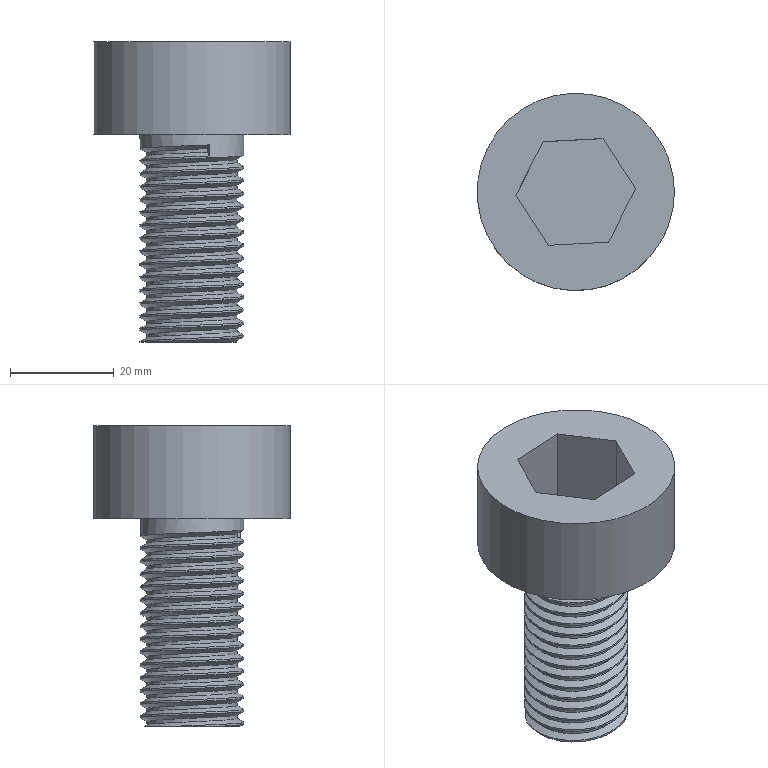Part | NX | features DATUM_CSYS 4, EXTRUDE 3, SKETCH 3, SYMBOLIC_THREAD 1, THREADS 1 | 1 solid | 31 faces | box 38 x 38 x 58 mm | volume 26254 mm3 | cylinder 18 | plane 11 | spline 2 | commonest cylinder face diameters 20 x16 17.5 x1 38 x1